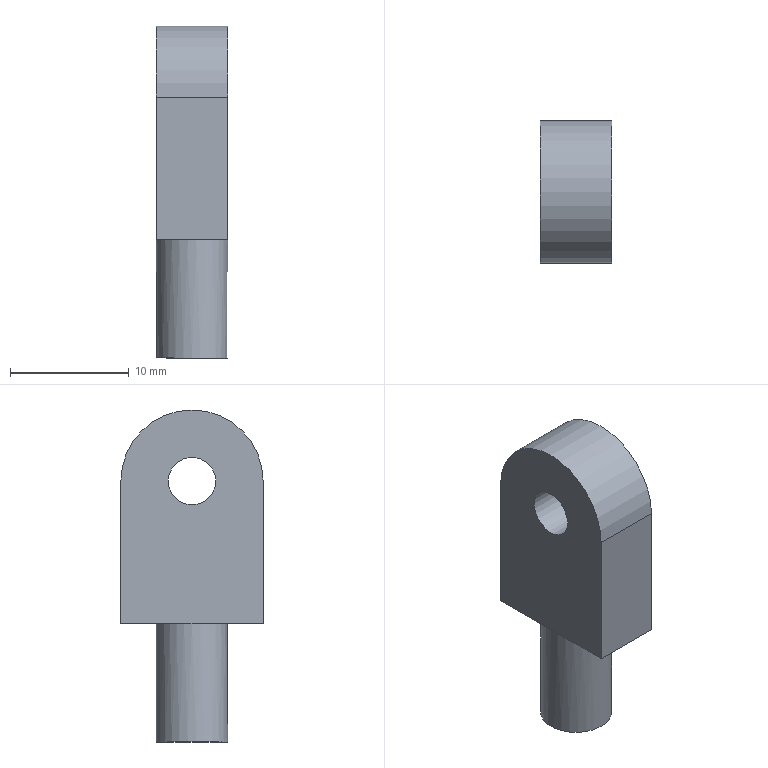Part | STEP file | 1-46.9 | 1 solid | 10 faces | box 6 x 12 x 28 mm | volume 1411 mm3 | plane 7 | cylinder 3 | commonest cylinder face diameters 4 x1 6 x1 12 x1
STEP:
#1=CARTESIAN_POINT('',(0.,0.,0.));
#2=DIRECTION('',(0.,0.,1.));
#3=DIRECTION('',(1.,0.,0.));
#4=AXIS2_PLACEMENT_3D('',#1,#2,#3);
#5=CARTESIAN_POINT('',(3.,6.,0.));
#6=VERTEX_POINT('',#5);
#7=CARTESIAN_POINT('',(3.,-6.,0.));
#8=VERTEX_POINT('',#7);
#9=CARTESIAN_POINT('',(3.,0.,0.));
#10=DIRECTION('',(1.,0.,0.));
#11=DIRECTION('',(0.,1.,0.));
#12=AXIS2_PLACEMENT_3D('',#9,#10,#11);
#13=CIRCLE('',#12,6.);
#14=CARTESIAN_POINT('',(3.,3.,-3.));
#15=DIRECTION('',(1.,0.,0.));
#16=DIRECTION('',(0.,1.,0.));
#17=AXIS2_PLACEMENT_3D('',#14,#15,#16);
#18=PLANE('',#17);
#19=CARTESIAN_POINT('',(-3.,3.));
#20=DIRECTION('',(1.,0.));
#21=AXIS2_PLACEMENT_2D('',#19,#20);
#22=CIRCLE('',#21,6.);
#23=(GEOMETRIC_REPRESENTATION_CONTEXT(2)PARAMETRIC_REPRESENTATION_CONTEXT()REPRESENTATION_CONTEXT('',''));
#24=DEFINITIONAL_REPRESENTATION('',(#22),#23);
#25=PCURVE('',#18,#24);
#26=CARTESIAN_POINT('',(3.,0.,0.));
#27=DIRECTION('',(-1.,0.,0.));
#28=DIRECTION('',(0.,1.,0.));
#29=AXIS2_PLACEMENT_3D('',#26,#27,#28);
#30=CYLINDRICAL_SURFACE('',#29,6.);
#31=CARTESIAN_POINT('',(6.283,0.));
#32=DIRECTION('',(-1.,0.));
#33=VECTOR('',#32,1.);
#34=LINE('',#31,#33);
#35=(GEOMETRIC_REPRESENTATION_CONTEXT(2)PARAMETRIC_REPRESENTATION_CONTEXT()REPRESENTATION_CONTEXT('',''));
#36=DEFINITIONAL_REPRESENTATION('',(#34),#35);
#37=PCURVE('',#30,#36);
#38=SURFACE_CURVE('',#13,(#25,#37),.PCURVE_S1.);
#39=EDGE_CURVE('',#6,#8,#38,.T.);
#40=ORIENTED_EDGE('',*,*,#39,.T.);
#41=CARTESIAN_POINT('',(3.,-6.,-12.));
#42=VERTEX_POINT('',#41);
#43=CARTESIAN_POINT('',(3.,-6.,0.));
#44=DIRECTION('',(0.,0.,-1.));
#45=VECTOR('',#44,1.);
#46=LINE('',#43,#45);
#47=CARTESIAN_POINT('',(-9.,3.));
#48=DIRECTION('',(0.,-1.));
#49=VECTOR('',#48,1.);
#50=LINE('',#47,#49);
#51=(GEOMETRIC_REPRESENTATION_CONTEXT(2)PARAMETRIC_REPRESENTATION_CONTEXT()REPRESENTATION_CONTEXT('',''));
#52=DEFINITIONAL_REPRESENTATION('',(#50),#51);
#53=PCURVE('',#18,#52);
#54=CARTESIAN_POINT('',(0.,-6.,-6.));
#55=DIRECTION('',(0.,1.,0.));
#56=DIRECTION('',(0.,0.,-1.));
#57=AXIS2_PLACEMENT_3D('',#54,#55,#56);
#58=PLANE('',#57);
#59=CARTESIAN_POINT('',(-6.,-3.));
#60=DIRECTION('',(1.,0.));
#61=VECTOR('',#60,1.);
#62=LINE('',#59,#61);
#63=(GEOMETRIC_REPRESENTATION_CONTEXT(2)PARAMETRIC_REPRESENTATION_CONTEXT()REPRESENTATION_CONTEXT('',''));
#64=DEFINITIONAL_REPRESENTATION('',(#62),#63);
#65=PCURVE('',#58,#64);
#66=SURFACE_CURVE('',#46,(#53,#65),.PCURVE_S1.);
#67=EDGE_CURVE('',#8,#42,#66,.T.);
#68=ORIENTED_EDGE('',*,*,#67,.T.);
#69=CARTESIAN_POINT('',(3.,0.,-12.));
#70=VERTEX_POINT('',#69);
#71=CARTESIAN_POINT('',(3.,-6.,-12.));
#72=DIRECTION('',(0.,1.,0.));
#73=VECTOR('',#72,1.);
#74=LINE('',#71,#73);
#75=CARTESIAN_POINT('',(-9.,-9.));
#76=DIRECTION('',(1.,0.));
#77=VECTOR('',#76,1.);
#78=LINE('',#75,#77);
#79=(GEOMETRIC_REPRESENTATION_CONTEXT(2)PARAMETRIC_REPRESENTATION_CONTEXT()REPRESENTATION_CONTEXT('',''));
#80=DEFINITIONAL_REPRESENTATION('',(#78),#79);
#81=PCURVE('',#18,#80);
#82=CARTESIAN_POINT('',(0.,0.,-12.));
#83=DIRECTION('',(0.,0.,1.));
#84=DIRECTION('',(0.,1.,0.));
#85=AXIS2_PLACEMENT_3D('',#82,#83,#84);
#86=PLANE('',#85);
#87=CARTESIAN_POINT('',(-6.,-3.));
#88=DIRECTION('',(1.,0.));
#89=VECTOR('',#88,1.);
#90=LINE('',#87,#89);
#91=(GEOMETRIC_REPRESENTATION_CONTEXT(2)PARAMETRIC_REPRESENTATION_CONTEXT()REPRESENTATION_CONTEXT('',''));
#92=DEFINITIONAL_REPRESENTATION('',(#90),#91);
#93=PCURVE('',#86,#92);
#94=SURFACE_CURVE('',#74,(#81,#93),.PCURVE_S1.);
#95=EDGE_CURVE('',#42,#70,#94,.T.);
#96=ORIENTED_EDGE('',*,*,#95,.T.);
#97=CARTESIAN_POINT('',(3.,6.,-12.));
#98=VERTEX_POINT('',#97);
#99=CARTESIAN_POINT('',(3.,0.,-12.));
#100=DIRECTION('',(0.,1.,0.));
#101=VECTOR('',#100,1.);
#102=LINE('',#99,#101);
#103=CARTESIAN_POINT('',(-3.,-9.));
#104=DIRECTION('',(1.,0.));
#105=VECTOR('',#104,1.);
#106=LINE('',#103,#105);
#107=(GEOMETRIC_REPRESENTATION_CONTEXT(2)PARAMETRIC_REPRESENTATION_CONTEXT()REPRESENTATION_CONTEXT('',''));
#108=DEFINITIONAL_REPRESENTATION('',(#106),#107);
#109=PCURVE('',#18,#108);
#110=CARTESIAN_POINT('',(0.,0.,-12.));
#111=DIRECTION('',(0.,0.,1.));
#112=DIRECTION('',(0.,1.,0.));
#113=AXIS2_PLACEMENT_3D('',#110,#111,#112);
#114=PLANE('',#113);
#115=CARTESIAN_POINT('',(0.,-3.));
#116=DIRECTION('',(1.,0.));
#117=VECTOR('',#116,1.);
#118=LINE('',#115,#117);
#119=(GEOMETRIC_REPRESENTATION_CONTEXT(2)PARAMETRIC_REPRESENTATION_CONTEXT()REPRESENTATION_CONTEXT('',''));
#120=DEFINITIONAL_REPRESENTATION('',(#118),#119);
#121=PCURVE('',#114,#120);
#122=SURFACE_CURVE('',#102,(#109,#121),.PCURVE_S1.);
#123=EDGE_CURVE('',#70,#98,#122,.T.);
#124=ORIENTED_EDGE('',*,*,#123,.T.);
#125=CARTESIAN_POINT('',(3.,6.,-12.));
#126=DIRECTION('',(0.,0.,1.));
#127=VECTOR('',#126,1.);
#128=LINE('',#125,#127);
#129=CARTESIAN_POINT('',(3.,-9.));
#130=DIRECTION('',(0.,1.));
#131=VECTOR('',#130,1.);
#132=LINE('',#129,#131);
#133=(GEOMETRIC_REPRESENTATION_CONTEXT(2)PARAMETRIC_REPRESENTATION_CONTEXT()REPRESENTATION_CONTEXT('',''));
#134=DEFINITIONAL_REPRESENTATION('',(#132),#133);
#135=PCURVE('',#18,#134);
#136=CARTESIAN_POINT('',(0.,6.,-6.));
#137=DIRECTION('',(0.,-1.,0.));
#138=DIRECTION('',(0.,0.,1.));
#139=AXIS2_PLACEMENT_3D('',#136,#137,#138);
#140=PLANE('',#139);
#141=CARTESIAN_POINT('',(-6.,-3.));
#142=DIRECTION('',(1.,0.));
#143=VECTOR('',#142,1.);
#144=LINE('',#141,#143);
#145=(GEOMETRIC_REPRESENTATION_CONTEXT(2)PARAMETRIC_REPRESENTATION_CONTEXT()REPRESENTATION_CONTEXT('',''));
#146=DEFINITIONAL_REPRESENTATION('',(#144),#145);
#147=PCURVE('',#140,#146);
#148=SURFACE_CURVE('',#128,(#135,#147),.PCURVE_S1.);
#149=EDGE_CURVE('',#98,#6,#148,.T.);
#150=ORIENTED_EDGE('',*,*,#149,.T.);
#151=EDGE_LOOP('',(#40,#68,#96,#124,#150));
#152=FACE_BOUND('',#151,.T.);
#153=CARTESIAN_POINT('',(3.,2.,0.));
#154=VERTEX_POINT('',#153);
#155=CARTESIAN_POINT('',(3.,0.,0.));
#156=DIRECTION('',(-1.,0.,0.));
#157=DIRECTION('',(0.,1.,0.));
#158=AXIS2_PLACEMENT_3D('',#155,#156,#157);
#159=CIRCLE('',#158,2.);
#160=CARTESIAN_POINT('',(-1.,3.));
#161=CARTESIAN_POINT('',(-1.,-0.4641));
#162=CARTESIAN_POINT('',(-4.,1.268));
#163=CARTESIAN_POINT('',(-7.,3.));
#164=CARTESIAN_POINT('',(-4.,4.732));
#165=CARTESIAN_POINT('',(-1.,6.464));
#166=CARTESIAN_POINT('',(-1.,3.));
#167=(BOUNDED_CURVE()B_SPLINE_CURVE(2,(#160,#161,#162,#163,#164,#165,#166),.UNSPECIFIED.,.T.,.F.)B_SPLINE_CURVE_WITH_KNOTS((1,2,2,2,2,1),(-2.094,0.,2.094,4.189,6.283,8.378),.UNSPECIFIED.)CURVE()GEOMETRIC_REPRESENTATION_ITEM()RATIONAL_B_SPLINE_CURVE((1.,0.5,1.,0.5,1.,0.5,1.))REPRESENTATION_ITEM(''));
#168=(GEOMETRIC_REPRESENTATION_CONTEXT(2)PARAMETRIC_REPRESENTATION_CONTEXT()REPRESENTATION_CONTEXT('',''));
#169=DEFINITIONAL_REPRESENTATION('',(#167),#168);
#170=PCURVE('',#18,#169);
#171=CARTESIAN_POINT('',(3.,0.,0.));
#172=DIRECTION('',(-1.,0.,0.));
#173=DIRECTION('',(0.,1.,0.));
#174=AXIS2_PLACEMENT_3D('',#171,#172,#173);
#175=CYLINDRICAL_SURFACE('',#174,2.);
#176=CARTESIAN_POINT('',(0.,0.));
#177=DIRECTION('',(1.,0.));
#178=VECTOR('',#177,1.);
#179=LINE('',#176,#178);
#180=(GEOMETRIC_REPRESENTATION_CONTEXT(2)PARAMETRIC_REPRESENTATION_CONTEXT()REPRESENTATION_CONTEXT('',''));
#181=DEFINITIONAL_REPRESENTATION('',(#179),#180);
#182=PCURVE('',#175,#181);
#183=SURFACE_CURVE('',#159,(#170,#182),.PCURVE_S1.);
#184=EDGE_CURVE('',#154,#154,#183,.T.);
#185=ORIENTED_EDGE('',*,*,#184,.T.);
#186=EDGE_LOOP('',(#185));
#187=FACE_BOUND('',#186,.T.);
#188=ADVANCED_FACE('',(#152,#187),#18,.T.);
#189=CARTESIAN_POINT('',(-3.,6.,0.));
#190=VERTEX_POINT('',#189);
#191=CARTESIAN_POINT('',(-3.,-6.,0.));
#192=VERTEX_POINT('',#191);
#193=CARTESIAN_POINT('',(-3.,0.,0.));
#194=DIRECTION('',(1.,0.,0.));
#195=DIRECTION('',(0.,1.,0.));
#196=AXIS2_PLACEMENT_3D('',#193,#194,#195);
#197=CIRCLE('',#196,6.);
#198=CARTESIAN_POINT('',(-3.,3.,-3.));
#199=DIRECTION('',(1.,0.,0.));
#200=DIRECTION('',(0.,1.,0.));
#201=AXIS2_PLACEMENT_3D('',#198,#199,#200);
#202=PLANE('',#201);
#203=CARTESIAN_POINT('',(-3.,3.));
#204=DIRECTION('',(1.,0.));
#205=AXIS2_PLACEMENT_2D('',#203,#204);
#206=CIRCLE('',#205,6.);
#207=(GEOMETRIC_REPRESENTATION_CONTEXT(2)PARAMETRIC_REPRESENTATION_CONTEXT()REPRESENTATION_CONTEXT('',''));
#208=DEFINITIONAL_REPRESENTATION('',(#206),#207);
#209=PCURVE('',#202,#208);
#210=CARTESIAN_POINT('',(6.283,6.));
#211=DIRECTION('',(-1.,0.));
#212=VECTOR('',#211,1.);
#213=LINE('',#210,#212);
#214=(GEOMETRIC_REPRESENTATION_CONTEXT(2)PARAMETRIC_REPRESENTATION_CONTEXT()REPRESENTATION_CONTEXT('',''));
#215=DEFINITIONAL_REPRESENTATION('',(#213),#214);
#216=PCURVE('',#30,#215);
#217=SURFACE_CURVE('',#197,(#209,#216),.PCURVE_S1.);
#218=EDGE_CURVE('',#190,#192,#217,.T.);
#219=ORIENTED_EDGE('',*,*,#218,.T.);
#220=CARTESIAN_POINT('',(-3.,-6.,-12.));
#221=VERTEX_POINT('',#220);
#222=CARTESIAN_POINT('',(-3.,-6.,0.));
#223=DIRECTION('',(0.,0.,-1.));
#224=VECTOR('',#223,1.);
#225=LINE('',#222,#224);
#226=CARTESIAN_POINT('',(-9.,3.));
#227=DIRECTION('',(0.,-1.));
#228=VECTOR('',#227,1.);
#229=LINE('',#226,#228);
#230=(GEOMETRIC_REPRESENTATION_CONTEXT(2)PARAMETRIC_REPRESENTATION_CONTEXT()REPRESENTATION_CONTEXT('',''));
#231=DEFINITIONAL_REPRESENTATION('',(#229),#230);
#232=PCURVE('',#202,#231);
#233=CARTESIAN_POINT('',(-6.,3.));
#234=DIRECTION('',(1.,0.));
#235=VECTOR('',#234,1.);
#236=LINE('',#233,#235);
#237=(GEOMETRIC_REPRESENTATION_CONTEXT(2)PARAMETRIC_REPRESENTATION_CONTEXT()REPRESENTATION_CONTEXT('',''));
#238=DEFINITIONAL_REPRESENTATION('',(#236),#237);
#239=PCURVE('',#58,#238);
#240=SURFACE_CURVE('',#225,(#232,#239),.PCURVE_S1.);
#241=EDGE_CURVE('',#192,#221,#240,.T.);
#242=ORIENTED_EDGE('',*,*,#241,.T.);
#243=CARTESIAN_POINT('',(-3.,0.,-12.));
#244=VERTEX_POINT('',#243);
#245=CARTESIAN_POINT('',(-3.,-6.,-12.));
#246=DIRECTION('',(0.,1.,0.));
#247=VECTOR('',#246,1.);
#248=LINE('',#245,#247);
#249=CARTESIAN_POINT('',(-9.,-9.));
#250=DIRECTION('',(1.,0.));
#251=VECTOR('',#250,1.);
#252=LINE('',#249,#251);
#253=(GEOMETRIC_REPRESENTATION_CONTEXT(2)PARAMETRIC_REPRESENTATION_CONTEXT()REPRESENTATION_CONTEXT('',''));
#254=DEFINITIONAL_REPRESENTATION('',(#252),#253);
#255=PCURVE('',#202,#254);
#256=CARTESIAN_POINT('',(-6.,3.));
#257=DIRECTION('',(1.,0.));
#258=VECTOR('',#257,1.);
#259=LINE('',#256,#258);
#260=(GEOMETRIC_REPRESENTATION_CONTEXT(2)PARAMETRIC_REPRESENTATION_CONTEXT()REPRESENTATION_CONTEXT('',''));
#261=DEFINITIONAL_REPRESENTATION('',(#259),#260);
#262=PCURVE('',#86,#261);
#263=SURFACE_CURVE('',#248,(#255,#262),.PCURVE_S1.);
#264=EDGE_CURVE('',#221,#244,#263,.T.);
#265=ORIENTED_EDGE('',*,*,#264,.T.);
#266=CARTESIAN_POINT('',(-3.,6.,-12.));
#267=VERTEX_POINT('',#266);
#268=CARTESIAN_POINT('',(-3.,0.,-12.));
#269=DIRECTION('',(0.,1.,0.));
#270=VECTOR('',#269,1.);
#271=LINE('',#268,#270);
#272=CARTESIAN_POINT('',(-3.,-9.));
#273=DIRECTION('',(1.,0.));
#274=VECTOR('',#273,1.);
#275=LINE('',#272,#274);
#276=(GEOMETRIC_REPRESENTATION_CONTEXT(2)PARAMETRIC_REPRESENTATION_CONTEXT()REPRESENTATION_CONTEXT('',''));
#277=DEFINITIONAL_REPRESENTATION('',(#275),#276);
#278=PCURVE('',#202,#277);
#279=CARTESIAN_POINT('',(0.,3.));
#280=DIRECTION('',(1.,0.));
#281=VECTOR('',#280,1.);
#282=LINE('',#279,#281);
#283=(GEOMETRIC_REPRESENTATION_CONTEXT(2)PARAMETRIC_REPRESENTATION_CONTEXT()REPRESENTATION_CONTEXT('',''));
#284=DEFINITIONAL_REPRESENTATION('',(#282),#283);
#285=PCURVE('',#114,#284);
#286=SURFACE_CURVE('',#271,(#278,#285),.PCURVE_S1.);
#287=EDGE_CURVE('',#244,#267,#286,.T.);
#288=ORIENTED_EDGE('',*,*,#287,.T.);
#289=CARTESIAN_POINT('',(-3.,6.,-12.));
#290=DIRECTION('',(0.,0.,1.));
#291=VECTOR('',#290,1.);
#292=LINE('',#289,#291);
#293=CARTESIAN_POINT('',(3.,-9.));
#294=DIRECTION('',(0.,1.));
#295=VECTOR('',#294,1.);
#296=LINE('',#293,#295);
#297=(GEOMETRIC_REPRESENTATION_CONTEXT(2)PARAMETRIC_REPRESENTATION_CONTEXT()REPRESENTATION_CONTEXT('',''));
#298=DEFINITIONAL_REPRESENTATION('',(#296),#297);
#299=PCURVE('',#202,#298);
#300=CARTESIAN_POINT('',(-6.,3.));
#301=DIRECTION('',(1.,0.));
#302=VECTOR('',#301,1.);
#303=LINE('',#300,#302);
#304=(GEOMETRIC_REPRESENTATION_CONTEXT(2)PARAMETRIC_REPRESENTATION_CONTEXT()REPRESENTATION_CONTEXT('',''));
#305=DEFINITIONAL_REPRESENTATION('',(#303),#304);
#306=PCURVE('',#140,#305);
#307=SURFACE_CURVE('',#292,(#299,#306),.PCURVE_S1.);
#308=EDGE_CURVE('',#267,#190,#307,.T.);
#309=ORIENTED_EDGE('',*,*,#308,.T.);
#310=EDGE_LOOP('',(#219,#242,#265,#288,#309));
#311=FACE_BOUND('',#310,.F.);
#312=CARTESIAN_POINT('',(-3.,2.,0.));
#313=VERTEX_POINT('',#312);
#314=CARTESIAN_POINT('',(-3.,0.,0.));
#315=DIRECTION('',(-1.,0.,0.));
#316=DIRECTION('',(0.,1.,0.));
#317=AXIS2_PLACEMENT_3D('',#314,#315,#316);
#318=CIRCLE('',#317,2.);
#319=CARTESIAN_POINT('',(-1.,3.));
#320=CARTESIAN_POINT('',(-1.,-0.4641));
#321=CARTESIAN_POINT('',(-4.,1.268));
#322=CARTESIAN_POINT('',(-7.,3.));
#323=CARTESIAN_POINT('',(-4.,4.732));
#324=CARTESIAN_POINT('',(-1.,6.464));
#325=CARTESIAN_POINT('',(-1.,3.));
#326=(BOUNDED_CURVE()B_SPLINE_CURVE(2,(#319,#320,#321,#322,#323,#324,#325),.UNSPECIFIED.,.T.,.F.)B_SPLINE_CURVE_WITH_KNOTS((1,2,2,2,2,1),(-2.094,0.,2.094,4.189,6.283,8.378),.UNSPECIFIED.)CURVE()GEOMETRIC_REPRESENTATION_ITEM()RATIONAL_B_SPLINE_CURVE((1.,0.5,1.,0.5,1.,0.5,1.))REPRESENTATION_ITEM(''));
#327=(GEOMETRIC_REPRESENTATION_CONTEXT(2)PARAMETRIC_REPRESENTATION_CONTEXT()REPRESENTATION_CONTEXT('',''));
#328=DEFINITIONAL_REPRESENTATION('',(#326),#327);
#329=PCURVE('',#202,#328);
#330=CARTESIAN_POINT('',(0.,6.));
#331=DIRECTION('',(1.,0.));
#332=VECTOR('',#331,1.);
#333=LINE('',#330,#332);
#334=(GEOMETRIC_REPRESENTATION_CONTEXT(2)PARAMETRIC_REPRESENTATION_CONTEXT()REPRESENTATION_CONTEXT('',''));
#335=DEFINITIONAL_REPRESENTATION('',(#333),#334);
#336=PCURVE('',#175,#335);
#337=SURFACE_CURVE('',#318,(#329,#336),.PCURVE_S1.);
#338=EDGE_CURVE('',#313,#313,#337,.T.);
#339=ORIENTED_EDGE('',*,*,#338,.T.);
#340=EDGE_LOOP('',(#339));
#341=FACE_BOUND('',#340,.F.);
#342=ADVANCED_FACE('',(#311,#341),#202,.F.);
#343=CARTESIAN_POINT('',(3.,6.,0.));
#344=DIRECTION('',(-1.,0.,0.));
#345=VECTOR('',#344,1.);
#346=LINE('',#343,#345);
#347=CARTESIAN_POINT('',(6.283,0.));
#348=DIRECTION('',(0.,1.));
#349=VECTOR('',#348,1.);
#350=LINE('',#347,#349);
#351=(GEOMETRIC_REPRESENTATION_CONTEXT(2)PARAMETRIC_REPRESENTATION_CONTEXT()REPRESENTATION_CONTEXT('',''));
#352=DEFINITIONAL_REPRESENTATION('',(#350),#351);
#353=PCURVE('',#30,#352);
#354=CARTESIAN_POINT('',(6.,-3.));
#355=DIRECTION('',(0.,1.));
#356=VECTOR('',#355,1.);
#357=LINE('',#354,#356);
#358=(GEOMETRIC_REPRESENTATION_CONTEXT(2)PARAMETRIC_REPRESENTATION_CONTEXT()REPRESENTATION_CONTEXT('',''));
#359=DEFINITIONAL_REPRESENTATION('',(#357),#358);
#360=PCURVE('',#140,#359);
#361=SURFACE_CURVE('',#346,(#353,#360),.PCURVE_S1.);
#362=EDGE_CURVE('',#6,#190,#361,.T.);
#363=ORIENTED_EDGE('',*,*,#362,.T.);
#364=ORIENTED_EDGE('',*,*,#218,.T.);
#365=CARTESIAN_POINT('',(3.,-6.,0.));
#366=DIRECTION('',(-1.,0.,0.));
#367=VECTOR('',#366,1.);
#368=LINE('',#365,#367);
#369=CARTESIAN_POINT('',(3.142,0.));
#370=DIRECTION('',(0.,1.));
#371=VECTOR('',#370,1.);
#372=LINE('',#369,#371);
#373=(GEOMETRIC_REPRESENTATION_CONTEXT(2)PARAMETRIC_REPRESENTATION_CONTEXT()REPRESENTATION_CONTEXT('',''));
#374=DEFINITIONAL_REPRESENTATION('',(#372),#373);
#375=PCURVE('',#30,#374);
#376=CARTESIAN_POINT('',(-6.,-3.));
#377=DIRECTION('',(0.,1.));
#378=VECTOR('',#377,1.);
#379=LINE('',#376,#378);
#380=(GEOMETRIC_REPRESENTATION_CONTEXT(2)PARAMETRIC_REPRESENTATION_CONTEXT()REPRESENTATION_CONTEXT('',''));
#381=DEFINITIONAL_REPRESENTATION('',(#379),#380);
#382=PCURVE('',#58,#381);
#383=SURFACE_CURVE('',#368,(#375,#382),.PCURVE_S1.);
#384=EDGE_CURVE('',#8,#192,#383,.T.);
#385=ORIENTED_EDGE('',*,*,#384,.F.);
#386=ORIENTED_EDGE('',*,*,#39,.F.);
#387=EDGE_LOOP('',(#363,#364,#385,#386));
#388=FACE_BOUND('',#387,.T.);
#389=ADVANCED_FACE('',(#388),#30,.T.);
#390=ORIENTED_EDGE('',*,*,#67,.T.);
#391=CARTESIAN_POINT('',(3.,-6.,-12.));
#392=DIRECTION('',(-1.,0.,0.));
#393=VECTOR('',#392,1.);
#394=LINE('',#391,#393);
#395=CARTESIAN_POINT('',(6.,-3.));
#396=DIRECTION('',(0.,1.));
#397=VECTOR('',#396,1.);
#398=LINE('',#395,#397);
#399=(GEOMETRIC_REPRESENTATION_CONTEXT(2)PARAMETRIC_REPRESENTATION_CONTEXT()REPRESENTATION_CONTEXT('',''));
#400=DEFINITIONAL_REPRESENTATION('',(#398),#399);
#401=PCURVE('',#58,#400);
#402=CARTESIAN_POINT('',(-6.,-3.));
#403=DIRECTION('',(0.,1.));
#404=VECTOR('',#403,1.);
#405=LINE('',#402,#404);
#406=(GEOMETRIC_REPRESENTATION_CONTEXT(2)PARAMETRIC_REPRESENTATION_CONTEXT()REPRESENTATION_CONTEXT('',''));
#407=DEFINITIONAL_REPRESENTATION('',(#405),#406);
#408=PCURVE('',#86,#407);
#409=SURFACE_CURVE('',#394,(#401,#408),.PCURVE_S1.);
#410=EDGE_CURVE('',#42,#221,#409,.T.);
#411=ORIENTED_EDGE('',*,*,#410,.T.);
#412=ORIENTED_EDGE('',*,*,#241,.F.);
#413=ORIENTED_EDGE('',*,*,#384,.F.);
#414=EDGE_LOOP('',(#390,#411,#412,#413));
#415=FACE_BOUND('',#414,.F.);
#416=ADVANCED_FACE('',(#415),#58,.F.);
#417=ORIENTED_EDGE('',*,*,#149,.T.);
#418=ORIENTED_EDGE('',*,*,#362,.T.);
#419=ORIENTED_EDGE('',*,*,#308,.F.);
#420=CARTESIAN_POINT('',(3.,6.,-12.));
#421=DIRECTION('',(-1.,0.,0.));
#422=VECTOR('',#421,1.);
#423=LINE('',#420,#422);
#424=CARTESIAN_POINT('',(-6.,-3.));
#425=DIRECTION('',(0.,1.));
#426=VECTOR('',#425,1.);
#427=LINE('',#424,#426);
#428=(GEOMETRIC_REPRESENTATION_CONTEXT(2)PARAMETRIC_REPRESENTATION_CONTEXT()REPRESENTATION_CONTEXT('',''));
#429=DEFINITIONAL_REPRESENTATION('',(#427),#428);
#430=PCURVE('',#140,#429);
#431=CARTESIAN_POINT('',(6.,-3.));
#432=DIRECTION('',(0.,1.));
#433=VECTOR('',#432,1.);
#434=LINE('',#431,#433);
#435=(GEOMETRIC_REPRESENTATION_CONTEXT(2)PARAMETRIC_REPRESENTATION_CONTEXT()REPRESENTATION_CONTEXT('',''));
#436=DEFINITIONAL_REPRESENTATION('',(#434),#435);
#437=PCURVE('',#114,#436);
#438=SURFACE_CURVE('',#423,(#430,#437),.PCURVE_S1.);
#439=EDGE_CURVE('',#98,#267,#438,.T.);
#440=ORIENTED_EDGE('',*,*,#439,.F.);
#441=EDGE_LOOP('',(#417,#418,#419,#440));
#442=FACE_BOUND('',#441,.F.);
#443=ADVANCED_FACE('',(#442),#140,.F.);
#444=ORIENTED_EDGE('',*,*,#184,.T.);
#445=CARTESIAN_POINT('',(3.,2.,0.));
#446=DIRECTION('',(-1.,0.,0.));
#447=VECTOR('',#446,1.);
#448=LINE('',#445,#447);
#449=CARTESIAN_POINT('',(6.283,0.));
#450=DIRECTION('',(0.,1.));
#451=VECTOR('',#450,1.);
#452=LINE('',#449,#451);
#453=(GEOMETRIC_REPRESENTATION_CONTEXT(2)PARAMETRIC_REPRESENTATION_CONTEXT()REPRESENTATION_CONTEXT('',''));
#454=DEFINITIONAL_REPRESENTATION('',(#452),#453);
#455=PCURVE('',#175,#454);
#456=CARTESIAN_POINT('',(0.,0.));
#457=DIRECTION('',(0.,1.));
#458=VECTOR('',#457,1.);
#459=LINE('',#456,#458);
#460=(GEOMETRIC_REPRESENTATION_CONTEXT(2)PARAMETRIC_REPRESENTATION_CONTEXT()REPRESENTATION_CONTEXT('',''));
#461=DEFINITIONAL_REPRESENTATION('',(#459),#460);
#462=PCURVE('',#175,#461);
#463=SEAM_CURVE('',#448,(#455,#462),.PCURVE_S1.);
#464=EDGE_CURVE('',#154,#313,#463,.T.);
#465=ORIENTED_EDGE('',*,*,#464,.T.);
#466=ORIENTED_EDGE('',*,*,#338,.F.);
#467=ORIENTED_EDGE('',*,*,#464,.F.);
#468=EDGE_LOOP('',(#444,#465,#466,#467));
#469=FACE_BOUND('',#468,.F.);
#470=ADVANCED_FACE('',(#469),#175,.F.);
#471=ORIENTED_EDGE('',*,*,#287,.F.);
#472=CARTESIAN_POINT('',(0.,3.,-12.));
#473=VERTEX_POINT('',#472);
#474=CARTESIAN_POINT('',(0.,0.,-12.));
#475=DIRECTION('',(0.,0.,-1.));
#476=DIRECTION('',(-1.,0.,0.));
#477=AXIS2_PLACEMENT_3D('',#474,#475,#476);
#478=CIRCLE('',#477,3.);
#479=CARTESIAN_POINT('',(0.,3.));
#480=CARTESIAN_POINT('',(5.196,3.));
#481=CARTESIAN_POINT('',(2.598,-1.5));
#482=CARTESIAN_POINT('',(0.,-6.));
#483=CARTESIAN_POINT('',(-2.598,-1.5));
#484=CARTESIAN_POINT('',(-5.196,3.));
#485=CARTESIAN_POINT('',(0.,3.));
#486=(BOUNDED_CURVE()B_SPLINE_CURVE(2,(#479,#480,#481,#482,#483,#484,#485),.UNSPECIFIED.,.T.,.F.)B_SPLINE_CURVE_WITH_KNOTS((1,2,2,2,2,1),(-2.094,0.,2.094,4.189,6.283,8.378),.UNSPECIFIED.)CURVE()GEOMETRIC_REPRESENTATION_ITEM()RATIONAL_B_SPLINE_CURVE((1.,0.5,1.,0.5,1.,0.5,1.))REPRESENTATION_ITEM(''));
#487=(GEOMETRIC_REPRESENTATION_CONTEXT(2)PARAMETRIC_REPRESENTATION_CONTEXT()REPRESENTATION_CONTEXT('',''));
#488=DEFINITIONAL_REPRESENTATION('',(#486),#487);
#489=PCURVE('',#114,#488);
#490=CARTESIAN_POINT('',(0.,0.,-12.));
#491=DIRECTION('',(0.,0.,-1.));
#492=DIRECTION('',(0.,1.,0.));
#493=AXIS2_PLACEMENT_3D('',#490,#491,#492);
#494=CYLINDRICAL_SURFACE('',#493,3.);
#495=CARTESIAN_POINT('',(4.712,0.));
#496=DIRECTION('',(1.,0.));
#497=VECTOR('',#496,1.);
#498=LINE('',#495,#497);
#499=(GEOMETRIC_REPRESENTATION_CONTEXT(2)PARAMETRIC_REPRESENTATION_CONTEXT()REPRESENTATION_CONTEXT('',''));
#500=DEFINITIONAL_REPRESENTATION('',(#498),#499);
#501=PCURVE('',#494,#500);
#502=SURFACE_CURVE('',#478,(#489,#501),.PCURVE_S1.);
#503=EDGE_CURVE('',#244,#473,#502,.T.);
#504=ORIENTED_EDGE('',*,*,#503,.T.);
#505=CARTESIAN_POINT('',(0.,0.,-12.));
#506=DIRECTION('',(0.,0.,-1.));
#507=DIRECTION('',(0.,1.,0.));
#508=AXIS2_PLACEMENT_3D('',#505,#506,#507);
#509=CIRCLE('',#508,3.);
#510=CARTESIAN_POINT('',(3.,0.));
#511=CARTESIAN_POINT('',(3.,-5.196));
#512=CARTESIAN_POINT('',(-1.5,-2.598));
#513=CARTESIAN_POINT('',(-6.,0.));
#514=CARTESIAN_POINT('',(-1.5,2.598));
#515=CARTESIAN_POINT('',(3.,5.196));
#516=CARTESIAN_POINT('',(3.,0.));
#517=(BOUNDED_CURVE()B_SPLINE_CURVE(2,(#510,#511,#512,#513,#514,#515,#516),.UNSPECIFIED.,.T.,.F.)B_SPLINE_CURVE_WITH_KNOTS((1,2,2,2,2,1),(-2.094,0.,2.094,4.189,6.283,8.378),.UNSPECIFIED.)CURVE()GEOMETRIC_REPRESENTATION_ITEM()RATIONAL_B_SPLINE_CURVE((1.,0.5,1.,0.5,1.,0.5,1.))REPRESENTATION_ITEM(''));
#518=(GEOMETRIC_REPRESENTATION_CONTEXT(2)PARAMETRIC_REPRESENTATION_CONTEXT()REPRESENTATION_CONTEXT('',''));
#519=DEFINITIONAL_REPRESENTATION('',(#517),#518);
#520=PCURVE('',#114,#519);
#521=CARTESIAN_POINT('',(0.,0.));
#522=DIRECTION('',(1.,0.));
#523=VECTOR('',#522,1.);
#524=LINE('',#521,#523);
#525=(GEOMETRIC_REPRESENTATION_CONTEXT(2)PARAMETRIC_REPRESENTATION_CONTEXT()REPRESENTATION_CONTEXT('',''));
#526=DEFINITIONAL_REPRESENTATION('',(#524),#525);
#527=PCURVE('',#494,#526);
#528=SURFACE_CURVE('',#509,(#520,#527),.PCURVE_S1.);
#529=EDGE_CURVE('',#473,#70,#528,.T.);
#530=ORIENTED_EDGE('',*,*,#529,.T.);
#531=ORIENTED_EDGE('',*,*,#123,.T.);
#532=ORIENTED_EDGE('',*,*,#439,.T.);
#533=EDGE_LOOP('',(#471,#504,#530,#531,#532));
#534=FACE_BOUND('',#533,.F.);
#535=ADVANCED_FACE('',(#534),#114,.F.);
#536=ORIENTED_EDGE('',*,*,#95,.T.);
#537=CARTESIAN_POINT('',(0.,0.,-12.));
#538=DIRECTION('',(0.,0.,-1.));
#539=DIRECTION('',(1.,0.,0.));
#540=AXIS2_PLACEMENT_3D('',#537,#538,#539);
#541=CIRCLE('',#540,3.);
#542=CARTESIAN_POINT('',(0.,-3.));
#543=CARTESIAN_POINT('',(-5.196,-3.));
#544=CARTESIAN_POINT('',(-2.598,1.5));
#545=CARTESIAN_POINT('',(0.,6.));
#546=CARTESIAN_POINT('',(2.598,1.5));
#547=CARTESIAN_POINT('',(5.196,-3.));
#548=CARTESIAN_POINT('',(0.,-3.));
#549=(BOUNDED_CURVE()B_SPLINE_CURVE(2,(#542,#543,#544,#545,#546,#547,#548),.UNSPECIFIED.,.T.,.F.)B_SPLINE_CURVE_WITH_KNOTS((1,2,2,2,2,1),(-2.094,0.,2.094,4.189,6.283,8.378),.UNSPECIFIED.)CURVE()GEOMETRIC_REPRESENTATION_ITEM()RATIONAL_B_SPLINE_CURVE((1.,0.5,1.,0.5,1.,0.5,1.))REPRESENTATION_ITEM(''));
#550=(GEOMETRIC_REPRESENTATION_CONTEXT(2)PARAMETRIC_REPRESENTATION_CONTEXT()REPRESENTATION_CONTEXT('',''));
#551=DEFINITIONAL_REPRESENTATION('',(#549),#550);
#552=PCURVE('',#86,#551);
#553=CARTESIAN_POINT('',(1.571,0.));
#554=DIRECTION('',(1.,0.));
#555=VECTOR('',#554,1.);
#556=LINE('',#553,#555);
#557=(GEOMETRIC_REPRESENTATION_CONTEXT(2)PARAMETRIC_REPRESENTATION_CONTEXT()REPRESENTATION_CONTEXT('',''));
#558=DEFINITIONAL_REPRESENTATION('',(#556),#557);
#559=PCURVE('',#494,#558);
#560=SURFACE_CURVE('',#541,(#552,#559),.PCURVE_S1.);
#561=EDGE_CURVE('',#70,#244,#560,.T.);
#562=ORIENTED_EDGE('',*,*,#561,.T.);
#563=ORIENTED_EDGE('',*,*,#264,.F.);
#564=ORIENTED_EDGE('',*,*,#410,.F.);
#565=EDGE_LOOP('',(#536,#562,#563,#564));
#566=FACE_BOUND('',#565,.F.);
#567=ADVANCED_FACE('',(#566),#86,.F.);
#568=ORIENTED_EDGE('',*,*,#529,.T.);
#569=ORIENTED_EDGE('',*,*,#561,.T.);
#570=ORIENTED_EDGE('',*,*,#503,.T.);
#571=CARTESIAN_POINT('',(0.,3.,-22.));
#572=VERTEX_POINT('',#571);
#573=CARTESIAN_POINT('',(0.,3.,-12.));
#574=DIRECTION('',(0.,0.,-1.));
#575=VECTOR('',#574,1.);
#576=LINE('',#573,#575);
#577=CARTESIAN_POINT('',(6.283,0.));
#578=DIRECTION('',(0.,1.));
#579=VECTOR('',#578,1.);
#580=LINE('',#577,#579);
#581=(GEOMETRIC_REPRESENTATION_CONTEXT(2)PARAMETRIC_REPRESENTATION_CONTEXT()REPRESENTATION_CONTEXT('',''));
#582=DEFINITIONAL_REPRESENTATION('',(#580),#581);
#583=PCURVE('',#494,#582);
#584=CARTESIAN_POINT('',(0.,0.));
#585=DIRECTION('',(0.,1.));
#586=VECTOR('',#585,1.);
#587=LINE('',#584,#586);
#588=(GEOMETRIC_REPRESENTATION_CONTEXT(2)PARAMETRIC_REPRESENTATION_CONTEXT()REPRESENTATION_CONTEXT('',''));
#589=DEFINITIONAL_REPRESENTATION('',(#587),#588);
#590=PCURVE('',#494,#589);
#591=SEAM_CURVE('',#576,(#583,#590),.PCURVE_S1.);
#592=EDGE_CURVE('',#473,#572,#591,.T.);
#593=ORIENTED_EDGE('',*,*,#592,.T.);
#594=CARTESIAN_POINT('',(0.,0.,-22.));
#595=DIRECTION('',(0.,0.,-1.));
#596=DIRECTION('',(0.,1.,0.));
#597=AXIS2_PLACEMENT_3D('',#594,#595,#596);
#598=CIRCLE('',#597,3.);
#599=CARTESIAN_POINT('',(0.,10.));
#600=DIRECTION('',(1.,0.));
#601=VECTOR('',#600,1.);
#602=LINE('',#599,#601);
#603=(GEOMETRIC_REPRESENTATION_CONTEXT(2)PARAMETRIC_REPRESENTATION_CONTEXT()REPRESENTATION_CONTEXT('',''));
#604=DEFINITIONAL_REPRESENTATION('',(#602),#603);
#605=PCURVE('',#494,#604);
#606=CARTESIAN_POINT('',(0.,-0.8038,-22.));
#607=DIRECTION('',(0.,0.,-1.));
#608=DIRECTION('',(0.,1.,0.));
#609=AXIS2_PLACEMENT_3D('',#606,#607,#608);
#610=PLANE('',#609);
#611=CARTESIAN_POINT('',(0.8038,0.));
#612=DIRECTION('',(1.,0.));
#613=AXIS2_PLACEMENT_2D('',#611,#612);
#614=CIRCLE('',#613,3.);
#615=(GEOMETRIC_REPRESENTATION_CONTEXT(2)PARAMETRIC_REPRESENTATION_CONTEXT()REPRESENTATION_CONTEXT('',''));
#616=DEFINITIONAL_REPRESENTATION('',(#614),#615);
#617=PCURVE('',#610,#616);
#618=SURFACE_CURVE('',#598,(#605,#617),.PCURVE_S1.);
#619=EDGE_CURVE('',#572,#572,#618,.T.);
#620=ORIENTED_EDGE('',*,*,#619,.F.);
#621=ORIENTED_EDGE('',*,*,#592,.F.);
#622=EDGE_LOOP('',(#568,#569,#570,#593,#620,#621));
#623=FACE_BOUND('',#622,.T.);
#624=ADVANCED_FACE('',(#623),#494,.T.);
#625=ORIENTED_EDGE('',*,*,#619,.T.);
#626=EDGE_LOOP('',(#625));
#627=FACE_BOUND('',#626,.T.);
#628=ADVANCED_FACE('',(#627),#610,.T.);
#629=CLOSED_SHELL('',(#188,#342,#389,#416,#443,#470,#535,#567,#624,#628));
#630=MANIFOLD_SOLID_BREP('',#629);
#631=(LENGTH_UNIT()NAMED_UNIT(*)SI_UNIT(.MILLI.,.METRE.));
#632=UNCERTAINTY_MEASURE_WITH_UNIT(LENGTH_MEASURE(0.0000001),#631,'','');
#633=(NAMED_UNIT(*)PLANE_ANGLE_UNIT()SI_UNIT($,.RADIAN.));
#634=(NAMED_UNIT(*)SI_UNIT($,.STERADIAN.)SOLID_ANGLE_UNIT());
#635=(GEOMETRIC_REPRESENTATION_CONTEXT(3)GLOBAL_UNCERTAINTY_ASSIGNED_CONTEXT((#632))GLOBAL_UNIT_ASSIGNED_CONTEXT((#631,#633,#634))REPRESENTATION_CONTEXT('',''));
#636=ADVANCED_BREP_SHAPE_REPRESENTATION('',(#4,#630),#635);